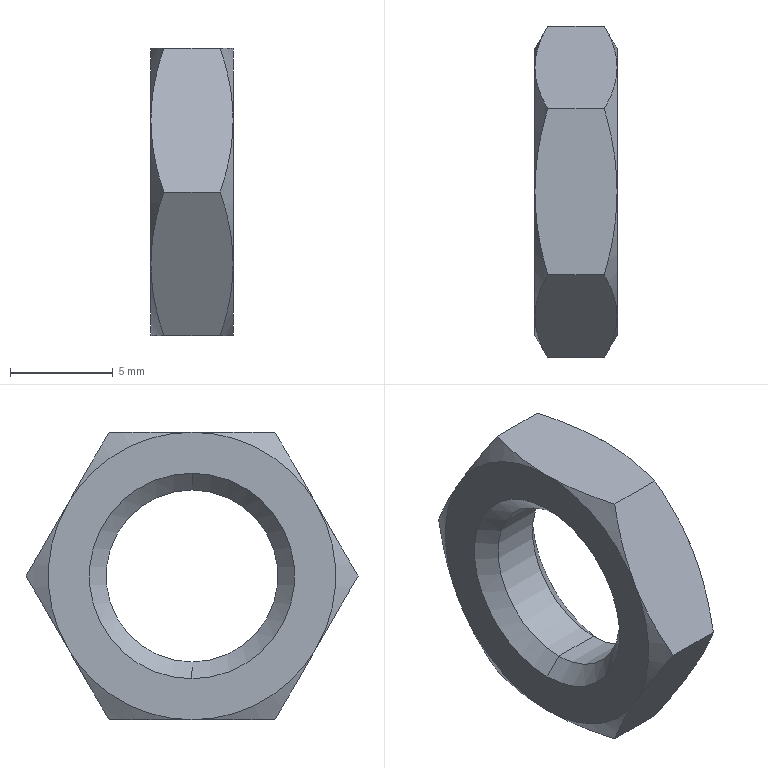Part | STEP file | 001-004-PB12nut | 1 solid | 26 faces | box 4 x 16.166 x 14 mm | volume 434.114 mm3 | cone 16 | plane 8 | cylinder 2 | commonest cylinder face diameters 8.376 x2